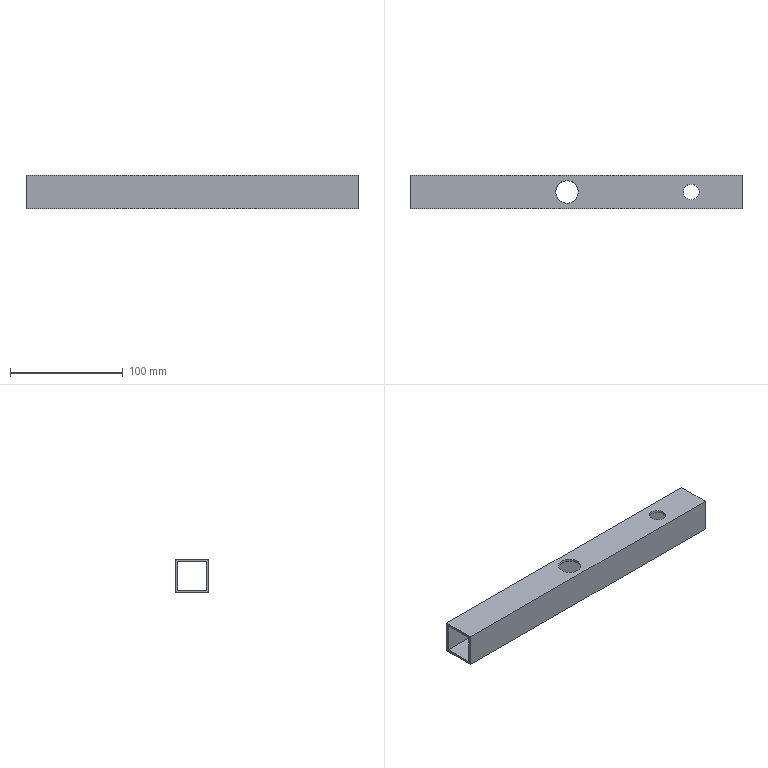Part | NX | features solid 2 | 1 solid | 14 faces | box 294.161 x 30 x 30 mm | volume 64020 mm3 | plane 10 | cylinder 4 | commonest cylinder face diameters 14 x2 20 x2
STEP:
#1=CARTESIAN_POINT('',(245.839,915.,-150.));
#2=VERTEX_POINT('',#1);
#3=CARTESIAN_POINT('',(540.,915.,-150.));
#4=VERTEX_POINT('',#3);
#5=CARTESIAN_POINT('',(335.,915.,-150.));
#6=DIRECTION('',(1.,0.,0.));
#7=VECTOR('',#6,1000.);
#8=LINE('',#5,#7);
#9=EDGE_CURVE('',#2,#4,#8,.T.);
#10=ORIENTED_EDGE('',*,*,#9,.F.);
#11=CARTESIAN_POINT('',(245.839,885.,-150.));
#12=VERTEX_POINT('',#11);
#13=CARTESIAN_POINT('',(245.839,916.,-150.));
#14=DIRECTION('',(0.,1.,0.));
#15=VECTOR('',#14,1000.);
#16=LINE('',#13,#15);
#17=EDGE_CURVE('',#2,#12,#16,.F.);
#18=ORIENTED_EDGE('',*,*,#17,.T.);
#19=CARTESIAN_POINT('',(540.,885.,-150.));
#20=VERTEX_POINT('',#19);
#21=CARTESIAN_POINT('',(335.,885.,-150.));
#22=DIRECTION('',(-1.,0.,0.));
#23=VECTOR('',#22,1000.);
#24=LINE('',#21,#23);
#25=EDGE_CURVE('',#12,#20,#24,.F.);
#26=ORIENTED_EDGE('',*,*,#25,.T.);
#27=CARTESIAN_POINT('',(540.,916.,-150.));
#28=DIRECTION('',(0.,-1.,0.));
#29=VECTOR('',#28,1000.);
#30=LINE('',#27,#29);
#31=EDGE_CURVE('',#4,#20,#30,.T.);
#32=ORIENTED_EDGE('',*,*,#31,.F.);
#33=EDGE_LOOP('',(#10,#18,#26,#32));
#34=FACE_BOUND('',#33,.T.);
#35=CARTESIAN_POINT('',(385.,910.,-150.));
#36=VERTEX_POINT('',#35);
#37=CARTESIAN_POINT('',(385.,900.,-150.));
#38=DIRECTION('',(0.,0.,1.));
#39=DIRECTION('',(0.,1.,0.));
#40=AXIS2_PLACEMENT_3D('',#37,#38,#39);
#41=CIRCLE('',#40,10.);
#42=EDGE_CURVE('',#36,#36,#41,.F.);
#43=ORIENTED_EDGE('',*,*,#42,.T.);
#44=EDGE_LOOP('',(#43));
#45=FACE_BOUND('',#44,.T.);
#46=CARTESIAN_POINT('',(495.,907.,-150.));
#47=VERTEX_POINT('',#46);
#48=CARTESIAN_POINT('',(495.,900.,-150.));
#49=DIRECTION('',(0.,0.,1.));
#50=DIRECTION('',(0.,1.,0.));
#51=AXIS2_PLACEMENT_3D('',#48,#49,#50);
#52=CIRCLE('',#51,7.);
#53=EDGE_CURVE('',#47,#47,#52,.F.);
#54=ORIENTED_EDGE('',*,*,#53,.T.);
#55=EDGE_LOOP('',(#54));
#56=FACE_BOUND('',#55,.T.);
#57=CARTESIAN_POINT('',(335.,916.,-150.));
#58=DIRECTION('',(0.,0.,1.));
#59=DIRECTION('',(0.,-1.,0.));
#60=AXIS2_PLACEMENT_3D('',#57,#58,#59);
#61=PLANE('',#60);
#62=ADVANCED_FACE('',(#34,#45,#56),#61,.T.);
#63=CARTESIAN_POINT('',(245.839,915.,-180.));
#64=VERTEX_POINT('',#63);
#65=CARTESIAN_POINT('',(245.839,885.,-180.));
#66=VERTEX_POINT('',#65);
#67=CARTESIAN_POINT('',(245.839,916.,-180.));
#68=DIRECTION('',(0.,1.,0.));
#69=VECTOR('',#68,1000.);
#70=LINE('',#67,#69);
#71=EDGE_CURVE('',#64,#66,#70,.F.);
#72=ORIENTED_EDGE('',*,*,#71,.F.);
#73=CARTESIAN_POINT('',(540.,915.,-180.));
#74=VERTEX_POINT('',#73);
#75=CARTESIAN_POINT('',(335.,915.,-180.));
#76=DIRECTION('',(1.,0.,0.));
#77=VECTOR('',#76,1000.);
#78=LINE('',#75,#77);
#79=EDGE_CURVE('',#64,#74,#78,.T.);
#80=ORIENTED_EDGE('',*,*,#79,.T.);
#81=CARTESIAN_POINT('',(540.,885.,-180.));
#82=VERTEX_POINT('',#81);
#83=CARTESIAN_POINT('',(540.,916.,-180.));
#84=DIRECTION('',(0.,-1.,0.));
#85=VECTOR('',#84,1000.);
#86=LINE('',#83,#85);
#87=EDGE_CURVE('',#74,#82,#86,.T.);
#88=ORIENTED_EDGE('',*,*,#87,.T.);
#89=CARTESIAN_POINT('',(335.,885.,-180.));
#90=DIRECTION('',(-1.,0.,0.));
#91=VECTOR('',#90,1000.);
#92=LINE('',#89,#91);
#93=EDGE_CURVE('',#66,#82,#92,.F.);
#94=ORIENTED_EDGE('',*,*,#93,.F.);
#95=EDGE_LOOP('',(#72,#80,#88,#94));
#96=FACE_BOUND('',#95,.T.);
#97=CARTESIAN_POINT('',(385.,910.,-180.));
#98=VERTEX_POINT('',#97);
#99=CARTESIAN_POINT('',(385.,900.,-180.));
#100=DIRECTION('',(0.,0.,1.));
#101=DIRECTION('',(0.,1.,0.));
#102=AXIS2_PLACEMENT_3D('',#99,#100,#101);
#103=CIRCLE('',#102,10.);
#104=EDGE_CURVE('',#98,#98,#103,.T.);
#105=ORIENTED_EDGE('',*,*,#104,.T.);
#106=EDGE_LOOP('',(#105));
#107=FACE_BOUND('',#106,.T.);
#108=CARTESIAN_POINT('',(495.,907.,-180.));
#109=VERTEX_POINT('',#108);
#110=CARTESIAN_POINT('',(495.,900.,-180.));
#111=DIRECTION('',(0.,0.,1.));
#112=DIRECTION('',(0.,1.,0.));
#113=AXIS2_PLACEMENT_3D('',#110,#111,#112);
#114=CIRCLE('',#113,7.);
#115=EDGE_CURVE('',#109,#109,#114,.T.);
#116=ORIENTED_EDGE('',*,*,#115,.T.);
#117=EDGE_LOOP('',(#116));
#118=FACE_BOUND('',#117,.T.);
#119=CARTESIAN_POINT('',(335.,916.,-180.));
#120=DIRECTION('',(0.,0.,1.));
#121=DIRECTION('',(0.,-1.,0.));
#122=AXIS2_PLACEMENT_3D('',#119,#120,#121);
#123=PLANE('',#122);
#124=ADVANCED_FACE('',(#96,#107,#118),#123,.F.);
#125=CARTESIAN_POINT('',(245.839,887.,-178.));
#126=VERTEX_POINT('',#125);
#127=CARTESIAN_POINT('',(245.839,913.,-178.));
#128=VERTEX_POINT('',#127);
#129=CARTESIAN_POINT('',(245.839,916.,-178.));
#130=DIRECTION('',(0.,-1.,0.));
#131=VECTOR('',#130,1000.);
#132=LINE('',#129,#131);
#133=EDGE_CURVE('',#126,#128,#132,.F.);
#134=ORIENTED_EDGE('',*,*,#133,.F.);
#135=CARTESIAN_POINT('',(540.,887.,-178.));
#136=VERTEX_POINT('',#135);
#137=CARTESIAN_POINT('',(760.,887.,-178.));
#138=DIRECTION('',(-1.,0.,0.));
#139=VECTOR('',#138,1000.);
#140=LINE('',#137,#139);
#141=EDGE_CURVE('',#136,#126,#140,.T.);
#142=ORIENTED_EDGE('',*,*,#141,.F.);
#143=CARTESIAN_POINT('',(540.,913.,-178.));
#144=VERTEX_POINT('',#143);
#145=CARTESIAN_POINT('',(540.,1064.528,-178.));
#146=DIRECTION('',(0.,-1.,0.));
#147=VECTOR('',#146,1000.);
#148=LINE('',#145,#147);
#149=EDGE_CURVE('',#144,#136,#148,.T.);
#150=ORIENTED_EDGE('',*,*,#149,.F.);
#151=CARTESIAN_POINT('',(760.,913.,-178.));
#152=DIRECTION('',(-1.,0.,0.));
#153=VECTOR('',#152,1000.);
#154=LINE('',#151,#153);
#155=EDGE_CURVE('',#144,#128,#154,.T.);
#156=ORIENTED_EDGE('',*,*,#155,.T.);
#157=EDGE_LOOP('',(#134,#142,#150,#156));
#158=FACE_BOUND('',#157,.T.);
#159=CARTESIAN_POINT('',(385.,890.,-178.));
#160=VERTEX_POINT('',#159);
#161=CARTESIAN_POINT('',(385.,900.,-178.));
#162=DIRECTION('',(0.,0.,-1.));
#163=DIRECTION('',(0.,-1.,0.));
#164=AXIS2_PLACEMENT_3D('',#161,#162,#163);
#165=CIRCLE('',#164,10.);
#166=EDGE_CURVE('',#160,#160,#165,.T.);
#167=ORIENTED_EDGE('',*,*,#166,.T.);
#168=EDGE_LOOP('',(#167));
#169=FACE_BOUND('',#168,.T.);
#170=CARTESIAN_POINT('',(495.,893.,-178.));
#171=VERTEX_POINT('',#170);
#172=CARTESIAN_POINT('',(495.,900.,-178.));
#173=DIRECTION('',(0.,0.,-1.));
#174=DIRECTION('',(0.,-1.,0.));
#175=AXIS2_PLACEMENT_3D('',#172,#173,#174);
#176=CIRCLE('',#175,7.);
#177=EDGE_CURVE('',#171,#171,#176,.F.);
#178=ORIENTED_EDGE('',*,*,#177,.F.);
#179=EDGE_LOOP('',(#178));
#180=FACE_BOUND('',#179,.T.);
#181=CARTESIAN_POINT('',(760.,916.,-178.));
#182=DIRECTION('',(0.,0.,-1.));
#183=DIRECTION('',(0.,1.,0.));
#184=AXIS2_PLACEMENT_3D('',#181,#182,#183);
#185=PLANE('',#184);
#186=ADVANCED_FACE('',(#158,#169,#180),#185,.F.);
#187=CARTESIAN_POINT('',(540.,887.,-152.));
#188=VERTEX_POINT('',#187);
#189=CARTESIAN_POINT('',(245.839,887.,-152.));
#190=VERTEX_POINT('',#189);
#191=CARTESIAN_POINT('',(760.,887.,-152.));
#192=DIRECTION('',(-1.,0.,0.));
#193=VECTOR('',#192,1000.);
#194=LINE('',#191,#193);
#195=EDGE_CURVE('',#188,#190,#194,.T.);
#196=ORIENTED_EDGE('',*,*,#195,.T.);
#197=CARTESIAN_POINT('',(245.839,913.,-152.));
#198=VERTEX_POINT('',#197);
#199=CARTESIAN_POINT('',(245.839,916.,-152.));
#200=DIRECTION('',(0.,-1.,0.));
#201=VECTOR('',#200,1000.);
#202=LINE('',#199,#201);
#203=EDGE_CURVE('',#190,#198,#202,.F.);
#204=ORIENTED_EDGE('',*,*,#203,.T.);
#205=CARTESIAN_POINT('',(540.,913.,-152.));
#206=VERTEX_POINT('',#205);
#207=CARTESIAN_POINT('',(760.,913.,-152.));
#208=DIRECTION('',(-1.,0.,0.));
#209=VECTOR('',#208,1000.);
#210=LINE('',#207,#209);
#211=EDGE_CURVE('',#206,#198,#210,.T.);
#212=ORIENTED_EDGE('',*,*,#211,.F.);
#213=CARTESIAN_POINT('',(540.,1064.528,-152.));
#214=DIRECTION('',(0.,-1.,0.));
#215=VECTOR('',#214,1000.);
#216=LINE('',#213,#215);
#217=EDGE_CURVE('',#206,#188,#216,.T.);
#218=ORIENTED_EDGE('',*,*,#217,.T.);
#219=EDGE_LOOP('',(#196,#204,#212,#218));
#220=FACE_BOUND('',#219,.T.);
#221=CARTESIAN_POINT('',(385.,890.,-152.));
#222=VERTEX_POINT('',#221);
#223=CARTESIAN_POINT('',(385.,900.,-152.));
#224=DIRECTION('',(0.,0.,-1.));
#225=DIRECTION('',(0.,-1.,0.));
#226=AXIS2_PLACEMENT_3D('',#223,#224,#225);
#227=CIRCLE('',#226,10.);
#228=EDGE_CURVE('',#222,#222,#227,.T.);
#229=ORIENTED_EDGE('',*,*,#228,.F.);
#230=EDGE_LOOP('',(#229));
#231=FACE_BOUND('',#230,.T.);
#232=CARTESIAN_POINT('',(495.,893.,-152.));
#233=VERTEX_POINT('',#232);
#234=CARTESIAN_POINT('',(495.,900.,-152.));
#235=DIRECTION('',(0.,0.,-1.));
#236=DIRECTION('',(0.,-1.,0.));
#237=AXIS2_PLACEMENT_3D('',#234,#235,#236);
#238=CIRCLE('',#237,7.);
#239=EDGE_CURVE('',#233,#233,#238,.F.);
#240=ORIENTED_EDGE('',*,*,#239,.T.);
#241=EDGE_LOOP('',(#240));
#242=FACE_BOUND('',#241,.T.);
#243=CARTESIAN_POINT('',(760.,916.,-152.));
#244=DIRECTION('',(0.,0.,-1.));
#245=DIRECTION('',(0.,1.,0.));
#246=AXIS2_PLACEMENT_3D('',#243,#244,#245);
#247=PLANE('',#246);
#248=ADVANCED_FACE('',(#220,#231,#242),#247,.T.);
#249=CARTESIAN_POINT('',(245.839,885.,-175.));
#250=DIRECTION('',(0.,0.,1.));
#251=VECTOR('',#250,1000.);
#252=LINE('',#249,#251);
#253=EDGE_CURVE('',#66,#12,#252,.T.);
#254=ORIENTED_EDGE('',*,*,#253,.F.);
#255=ORIENTED_EDGE('',*,*,#93,.T.);
#256=CARTESIAN_POINT('',(540.,885.,-160.));
#257=DIRECTION('',(0.,0.,1.));
#258=VECTOR('',#257,1000.);
#259=LINE('',#256,#258);
#260=EDGE_CURVE('',#20,#82,#259,.F.);
#261=ORIENTED_EDGE('',*,*,#260,.F.);
#262=ORIENTED_EDGE('',*,*,#25,.F.);
#263=EDGE_LOOP('',(#254,#255,#261,#262));
#264=FACE_BOUND('',#263,.T.);
#265=CARTESIAN_POINT('',(335.,885.,-175.));
#266=DIRECTION('',(0.,-1.,0.));
#267=DIRECTION('',(1.,0.,0.));
#268=AXIS2_PLACEMENT_3D('',#265,#266,#267);
#269=PLANE('',#268);
#270=ADVANCED_FACE('',(#264),#269,.T.);
#271=CARTESIAN_POINT('',(245.839,915.,-175.));
#272=DIRECTION('',(0.,0.,1.));
#273=VECTOR('',#272,1000.);
#274=LINE('',#271,#273);
#275=EDGE_CURVE('',#2,#64,#274,.F.);
#276=ORIENTED_EDGE('',*,*,#275,.F.);
#277=ORIENTED_EDGE('',*,*,#9,.T.);
#278=CARTESIAN_POINT('',(540.,915.,-175.));
#279=DIRECTION('',(0.,0.,-1.));
#280=VECTOR('',#279,1000.);
#281=LINE('',#278,#280);
#282=EDGE_CURVE('',#4,#74,#281,.T.);
#283=ORIENTED_EDGE('',*,*,#282,.T.);
#284=ORIENTED_EDGE('',*,*,#79,.F.);
#285=EDGE_LOOP('',(#276,#277,#283,#284));
#286=FACE_BOUND('',#285,.T.);
#287=CARTESIAN_POINT('',(335.,915.,-175.));
#288=DIRECTION('',(0.,-1.,0.));
#289=DIRECTION('',(1.,0.,0.));
#290=AXIS2_PLACEMENT_3D('',#287,#288,#289);
#291=PLANE('',#290);
#292=ADVANCED_FACE('',(#286),#291,.F.);
#293=CARTESIAN_POINT('',(245.839,913.,-175.));
#294=DIRECTION('',(0.,0.,-1.));
#295=VECTOR('',#294,1000.);
#296=LINE('',#293,#295);
#297=EDGE_CURVE('',#128,#198,#296,.F.);
#298=ORIENTED_EDGE('',*,*,#297,.F.);
#299=ORIENTED_EDGE('',*,*,#155,.F.);
#300=CARTESIAN_POINT('',(540.,913.,-160.));
#301=DIRECTION('',(0.,0.,-1.));
#302=VECTOR('',#301,1000.);
#303=LINE('',#300,#302);
#304=EDGE_CURVE('',#206,#144,#303,.T.);
#305=ORIENTED_EDGE('',*,*,#304,.F.);
#306=ORIENTED_EDGE('',*,*,#211,.T.);
#307=EDGE_LOOP('',(#298,#299,#305,#306));
#308=FACE_BOUND('',#307,.T.);
#309=CARTESIAN_POINT('',(760.,913.,-175.));
#310=DIRECTION('',(0.,1.,0.));
#311=DIRECTION('',(0.,0.,1.));
#312=AXIS2_PLACEMENT_3D('',#309,#310,#311);
#313=PLANE('',#312);
#314=ADVANCED_FACE('',(#308),#313,.F.);
#315=ORIENTED_EDGE('',*,*,#141,.T.);
#316=CARTESIAN_POINT('',(245.839,887.,-175.));
#317=DIRECTION('',(0.,0.,-1.));
#318=VECTOR('',#317,1000.);
#319=LINE('',#316,#318);
#320=EDGE_CURVE('',#126,#190,#319,.F.);
#321=ORIENTED_EDGE('',*,*,#320,.T.);
#322=ORIENTED_EDGE('',*,*,#195,.F.);
#323=CARTESIAN_POINT('',(540.,887.,-160.));
#324=DIRECTION('',(0.,0.,-1.));
#325=VECTOR('',#324,1000.);
#326=LINE('',#323,#325);
#327=EDGE_CURVE('',#188,#136,#326,.T.);
#328=ORIENTED_EDGE('',*,*,#327,.T.);
#329=EDGE_LOOP('',(#315,#321,#322,#328));
#330=FACE_BOUND('',#329,.T.);
#331=CARTESIAN_POINT('',(760.,887.,-175.));
#332=DIRECTION('',(0.,1.,0.));
#333=DIRECTION('',(0.,0.,1.));
#334=AXIS2_PLACEMENT_3D('',#331,#332,#333);
#335=PLANE('',#334);
#336=ADVANCED_FACE('',(#330),#335,.T.);
#337=ORIENTED_EDGE('',*,*,#42,.F.);
#338=EDGE_LOOP('',(#337));
#339=FACE_BOUND('',#338,.T.);
#340=ORIENTED_EDGE('',*,*,#228,.T.);
#341=EDGE_LOOP('',(#340));
#342=FACE_BOUND('',#341,.T.);
#343=CARTESIAN_POINT('',(385.,900.,-122.));
#344=DIRECTION('',(0.,0.,-1.));
#345=DIRECTION('',(0.,1.,0.));
#346=AXIS2_PLACEMENT_3D('',#343,#344,#345);
#347=CYLINDRICAL_SURFACE('',#346,10.);
#348=ADVANCED_FACE('',(#339,#342),#347,.F.);
#349=ORIENTED_EDGE('',*,*,#217,.F.);
#350=ORIENTED_EDGE('',*,*,#304,.T.);
#351=ORIENTED_EDGE('',*,*,#149,.T.);
#352=ORIENTED_EDGE('',*,*,#327,.F.);
#353=EDGE_LOOP('',(#349,#350,#351,#352));
#354=FACE_BOUND('',#353,.T.);
#355=ORIENTED_EDGE('',*,*,#260,.T.);
#356=ORIENTED_EDGE('',*,*,#87,.F.);
#357=ORIENTED_EDGE('',*,*,#282,.F.);
#358=ORIENTED_EDGE('',*,*,#31,.T.);
#359=EDGE_LOOP('',(#355,#356,#357,#358));
#360=FACE_BOUND('',#359,.T.);
#361=CARTESIAN_POINT('',(540.,1064.528,-160.));
#362=DIRECTION('',(-1.,0.,0.));
#363=DIRECTION('',(0.,0.,1.));
#364=AXIS2_PLACEMENT_3D('',#361,#362,#363);
#365=PLANE('',#364);
#366=ADVANCED_FACE('',(#354,#360),#365,.F.);
#367=ORIENTED_EDGE('',*,*,#166,.F.);
#368=EDGE_LOOP('',(#367));
#369=FACE_BOUND('',#368,.T.);
#370=ORIENTED_EDGE('',*,*,#104,.F.);
#371=EDGE_LOOP('',(#370));
#372=FACE_BOUND('',#371,.T.);
#373=CARTESIAN_POINT('',(385.,900.,-122.));
#374=DIRECTION('',(0.,0.,-1.));
#375=DIRECTION('',(0.,1.,0.));
#376=AXIS2_PLACEMENT_3D('',#373,#374,#375);
#377=CYLINDRICAL_SURFACE('',#376,10.);
#378=ADVANCED_FACE('',(#369,#372),#377,.F.);
#379=ORIENTED_EDGE('',*,*,#320,.F.);
#380=ORIENTED_EDGE('',*,*,#133,.T.);
#381=ORIENTED_EDGE('',*,*,#297,.T.);
#382=ORIENTED_EDGE('',*,*,#203,.F.);
#383=EDGE_LOOP('',(#379,#380,#381,#382));
#384=FACE_BOUND('',#383,.T.);
#385=ORIENTED_EDGE('',*,*,#71,.T.);
#386=ORIENTED_EDGE('',*,*,#253,.T.);
#387=ORIENTED_EDGE('',*,*,#17,.F.);
#388=ORIENTED_EDGE('',*,*,#275,.T.);
#389=EDGE_LOOP('',(#385,#386,#387,#388));
#390=FACE_BOUND('',#389,.T.);
#391=CARTESIAN_POINT('',(245.839,776.479,-210.));
#392=DIRECTION('',(1.,0.,0.));
#393=DIRECTION('',(0.,1.,0.));
#394=AXIS2_PLACEMENT_3D('',#391,#392,#393);
#395=PLANE('',#394);
#396=ADVANCED_FACE('',(#384,#390),#395,.F.);
#397=ORIENTED_EDGE('',*,*,#53,.F.);
#398=EDGE_LOOP('',(#397));
#399=FACE_BOUND('',#398,.T.);
#400=ORIENTED_EDGE('',*,*,#239,.F.);
#401=EDGE_LOOP('',(#400));
#402=FACE_BOUND('',#401,.T.);
#403=CARTESIAN_POINT('',(495.,900.,-175.));
#404=DIRECTION('',(0.,0.,-1.));
#405=DIRECTION('',(0.,1.,0.));
#406=AXIS2_PLACEMENT_3D('',#403,#404,#405);
#407=CYLINDRICAL_SURFACE('',#406,7.);
#408=ADVANCED_FACE('',(#399,#402),#407,.F.);
#409=ORIENTED_EDGE('',*,*,#115,.F.);
#410=EDGE_LOOP('',(#409));
#411=FACE_BOUND('',#410,.T.);
#412=ORIENTED_EDGE('',*,*,#177,.T.);
#413=EDGE_LOOP('',(#412));
#414=FACE_BOUND('',#413,.T.);
#415=CARTESIAN_POINT('',(495.,900.,-175.));
#416=DIRECTION('',(0.,0.,-1.));
#417=DIRECTION('',(0.,1.,0.));
#418=AXIS2_PLACEMENT_3D('',#415,#416,#417);
#419=CYLINDRICAL_SURFACE('',#418,7.);
#420=ADVANCED_FACE('',(#411,#414),#419,.F.);
#421=CLOSED_SHELL('',(#62,#124,#186,#248,#270,#292,#314,#336,#348,#366,#378,#396,#408,#420));
#422=MANIFOLD_SOLID_BREP('',#421);
#423=(LENGTH_UNIT()NAMED_UNIT(*)SI_UNIT(.MILLI.,.METRE.));
#424=UNCERTAINTY_MEASURE_WITH_UNIT(LENGTH_MEASURE(0.00001),#423,'','');
#425=(NAMED_UNIT(*)PLANE_ANGLE_UNIT()SI_UNIT($,.RADIAN.));
#426=(NAMED_UNIT(*)SI_UNIT($,.STERADIAN.)SOLID_ANGLE_UNIT());
#427=(GEOMETRIC_REPRESENTATION_CONTEXT(3)GLOBAL_UNCERTAINTY_ASSIGNED_CONTEXT((#424))GLOBAL_UNIT_ASSIGNED_CONTEXT((#423,#425,#426))REPRESENTATION_CONTEXT('',''));
#428=ADVANCED_BREP_SHAPE_REPRESENTATION('',(#422),#427);